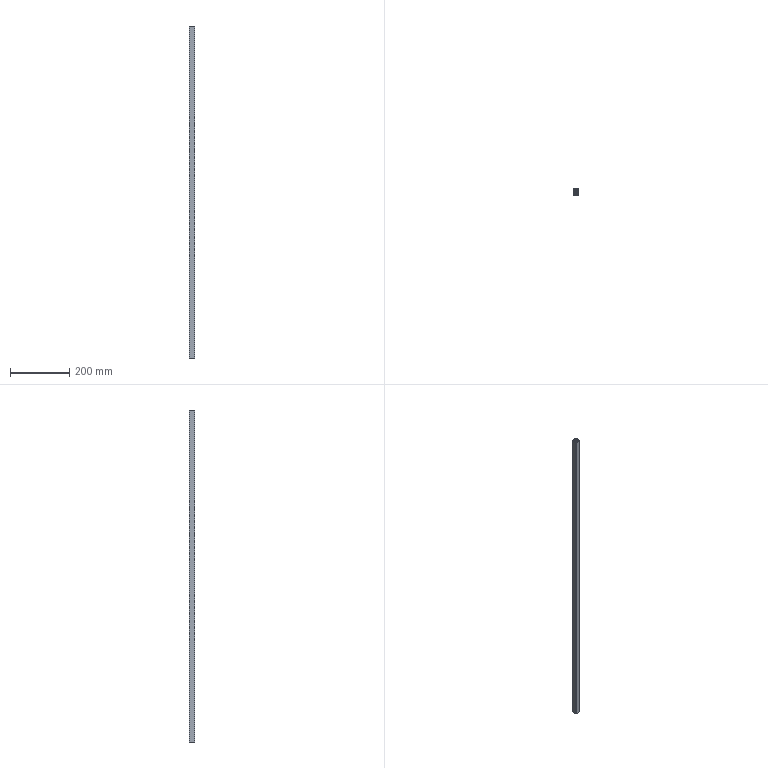Part | 1 solid | 72 faces | box 20 x 20 x 1125 mm | volume 221320 mm3 | plane 38 | cylinder 34 | commonest cylinder face diameters 0.6 x20 4 x8 3 x4 5 x2